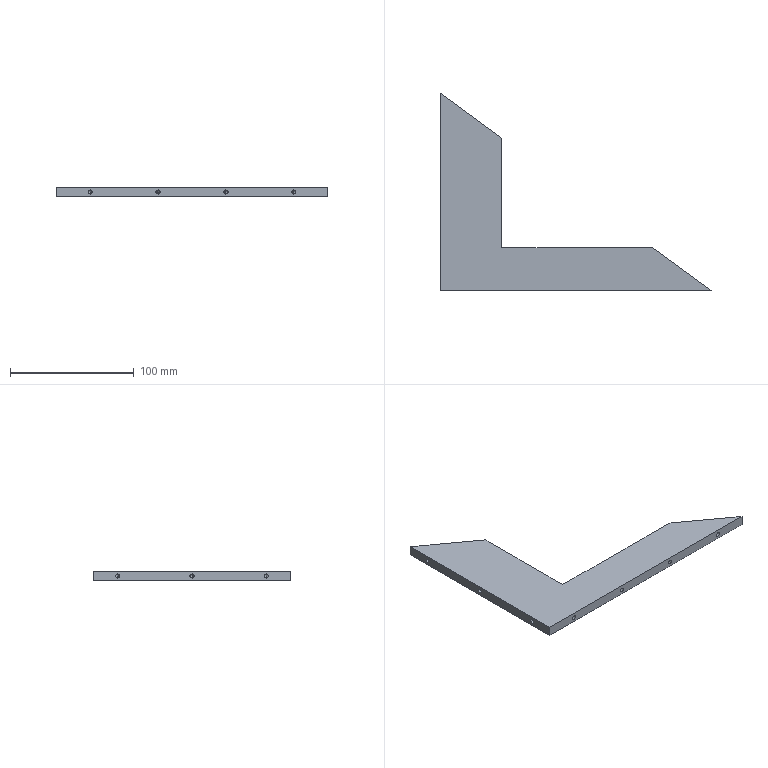Part | SolidWorks | features HoleWzd 2, Extrusion 1 | 1 solid | 36 faces | box 220 x 160 x 8 mm | volume 96669 mm3 | cylinder 14 | cone 14 | plane 8 | commonest cylinder face diameters 3.3 x14
STEP:
#1=CARTESIAN_POINT('',(-124.9,20.,2.35));
#2=VERTEX_POINT('',#1);
#3=CARTESIAN_POINT('',(-124.9,20.,5.65));
#4=VERTEX_POINT('',#3);
#5=CARTESIAN_POINT('',(-124.9,20.,4.));
#6=DIRECTION('',(-1.,0.,0.));
#7=DIRECTION('',(0.,0.,1.));
#8=AXIS2_PLACEMENT_3D('',#5,#6,#7);
#9=CIRCLE('',#8,1.65);
#10=EDGE_CURVE('',#2,#4,#9,.T.);
#11=ORIENTED_EDGE('',*,*,#10,.F.);
#12=CARTESIAN_POINT('',(-140.,20.,2.35));
#13=VERTEX_POINT('',#12);
#14=CARTESIAN_POINT('',(-140.,20.,2.35));
#15=DIRECTION('',(-1.,0.,0.));
#16=VECTOR('',#15,1000.);
#17=LINE('',#14,#16);
#18=EDGE_CURVE('',#2,#13,#17,.T.);
#19=ORIENTED_EDGE('',*,*,#18,.T.);
#20=CARTESIAN_POINT('',(-140.,20.,5.65));
#21=VERTEX_POINT('',#20);
#22=CARTESIAN_POINT('',(-140.,20.,4.));
#23=DIRECTION('',(-1.,0.,0.));
#24=DIRECTION('',(0.,0.,1.));
#25=AXIS2_PLACEMENT_3D('',#22,#23,#24);
#26=CIRCLE('',#25,1.65);
#27=EDGE_CURVE('',#13,#21,#26,.T.);
#28=ORIENTED_EDGE('',*,*,#27,.T.);
#29=CARTESIAN_POINT('',(-140.,20.,5.65));
#30=DIRECTION('',(-1.,0.,0.));
#31=VECTOR('',#30,1000.);
#32=LINE('',#29,#31);
#33=EDGE_CURVE('',#4,#21,#32,.T.);
#34=ORIENTED_EDGE('',*,*,#33,.F.);
#35=EDGE_LOOP('',(#11,#19,#28,#34));
#36=FACE_OUTER_BOUND('',#35,.T.);
#37=CARTESIAN_POINT('',(-140.,20.,4.));
#38=DIRECTION('',(-1.,0.,0.));
#39=DIRECTION('',(0.,0.,1.));
#40=AXIS2_PLACEMENT_3D('',#37,#38,#39);
#41=CYLINDRICAL_SURFACE('',#40,1.65);
#42=ADVANCED_FACE('',(#36),#41,.F.);
#43=CARTESIAN_POINT('',(-123.909,20.,4.));
#44=VERTEX_POINT('',#43);
#45=CARTESIAN_POINT('',(-124.9,20.,5.65));
#46=DIRECTION('',(-0.515,0.,0.8572));
#47=VECTOR('',#46,1000.);
#48=LINE('',#45,#47);
#49=EDGE_CURVE('',#44,#4,#48,.T.);
#50=ORIENTED_EDGE('',*,*,#49,.F.);
#51=CARTESIAN_POINT('',(-124.9,20.,2.35));
#52=DIRECTION('',(-0.515,0.,-0.8572));
#53=VECTOR('',#52,1000.);
#54=LINE('',#51,#53);
#55=EDGE_CURVE('',#44,#2,#54,.T.);
#56=ORIENTED_EDGE('',*,*,#55,.T.);
#57=ORIENTED_EDGE('',*,*,#10,.T.);
#58=EDGE_LOOP('',(#50,#56,#57));
#59=FACE_OUTER_BOUND('',#58,.T.);
#60=CARTESIAN_POINT('',(-124.9,20.,4.));
#61=DIRECTION('',(-1.,0.,0.));
#62=DIRECTION('',(0.,0.,1.));
#63=AXIS2_PLACEMENT_3D('',#60,#61,#62);
#64=CONICAL_SURFACE('',#63,1.65,1.03);
#65=ADVANCED_FACE('',(#59),#64,.F.);
#66=CARTESIAN_POINT('',(-124.9,-40.,2.35));
#67=VERTEX_POINT('',#66);
#68=CARTESIAN_POINT('',(-124.9,-40.,5.65));
#69=VERTEX_POINT('',#68);
#70=CARTESIAN_POINT('',(-124.9,-40.,4.));
#71=DIRECTION('',(-1.,0.,0.));
#72=DIRECTION('',(0.,0.,1.));
#73=AXIS2_PLACEMENT_3D('',#70,#71,#72);
#74=CIRCLE('',#73,1.65);
#75=EDGE_CURVE('',#67,#69,#74,.T.);
#76=ORIENTED_EDGE('',*,*,#75,.F.);
#77=CARTESIAN_POINT('',(-140.,-40.,2.35));
#78=VERTEX_POINT('',#77);
#79=CARTESIAN_POINT('',(-140.,-40.,2.35));
#80=DIRECTION('',(-1.,0.,0.));
#81=VECTOR('',#80,1000.);
#82=LINE('',#79,#81);
#83=EDGE_CURVE('',#67,#78,#82,.T.);
#84=ORIENTED_EDGE('',*,*,#83,.T.);
#85=CARTESIAN_POINT('',(-140.,-40.,5.65));
#86=VERTEX_POINT('',#85);
#87=CARTESIAN_POINT('',(-140.,-40.,4.));
#88=DIRECTION('',(-1.,0.,0.));
#89=DIRECTION('',(0.,0.,1.));
#90=AXIS2_PLACEMENT_3D('',#87,#88,#89);
#91=CIRCLE('',#90,1.65);
#92=EDGE_CURVE('',#78,#86,#91,.T.);
#93=ORIENTED_EDGE('',*,*,#92,.T.);
#94=CARTESIAN_POINT('',(-140.,-40.,5.65));
#95=DIRECTION('',(-1.,0.,0.));
#96=VECTOR('',#95,1000.);
#97=LINE('',#94,#96);
#98=EDGE_CURVE('',#69,#86,#97,.T.);
#99=ORIENTED_EDGE('',*,*,#98,.F.);
#100=EDGE_LOOP('',(#76,#84,#93,#99));
#101=FACE_OUTER_BOUND('',#100,.T.);
#102=CARTESIAN_POINT('',(-140.,-40.,4.));
#103=DIRECTION('',(-1.,0.,0.));
#104=DIRECTION('',(0.,0.,1.));
#105=AXIS2_PLACEMENT_3D('',#102,#103,#104);
#106=CYLINDRICAL_SURFACE('',#105,1.65);
#107=ADVANCED_FACE('',(#101),#106,.F.);
#108=CARTESIAN_POINT('',(-123.909,-40.,4.));
#109=VERTEX_POINT('',#108);
#110=CARTESIAN_POINT('',(-124.9,-40.,5.65));
#111=DIRECTION('',(-0.515,0.,0.8572));
#112=VECTOR('',#111,1000.);
#113=LINE('',#110,#112);
#114=EDGE_CURVE('',#109,#69,#113,.T.);
#115=ORIENTED_EDGE('',*,*,#114,.F.);
#116=CARTESIAN_POINT('',(-124.9,-40.,2.35));
#117=DIRECTION('',(-0.515,0.,-0.8572));
#118=VECTOR('',#117,1000.);
#119=LINE('',#116,#118);
#120=EDGE_CURVE('',#109,#67,#119,.T.);
#121=ORIENTED_EDGE('',*,*,#120,.T.);
#122=ORIENTED_EDGE('',*,*,#75,.T.);
#123=EDGE_LOOP('',(#115,#121,#122));
#124=FACE_OUTER_BOUND('',#123,.T.);
#125=CARTESIAN_POINT('',(-124.9,-40.,4.));
#126=DIRECTION('',(-1.,0.,0.));
#127=DIRECTION('',(0.,0.,1.));
#128=AXIS2_PLACEMENT_3D('',#125,#126,#127);
#129=CONICAL_SURFACE('',#128,1.65,1.03);
#130=ADVANCED_FACE('',(#124),#129,.F.);
#131=CARTESIAN_POINT('',(-124.9,-100.,2.35));
#132=VERTEX_POINT('',#131);
#133=CARTESIAN_POINT('',(-124.9,-100.,5.65));
#134=VERTEX_POINT('',#133);
#135=CARTESIAN_POINT('',(-124.9,-100.,4.));
#136=DIRECTION('',(-1.,0.,0.));
#137=DIRECTION('',(0.,0.,1.));
#138=AXIS2_PLACEMENT_3D('',#135,#136,#137);
#139=CIRCLE('',#138,1.65);
#140=EDGE_CURVE('',#132,#134,#139,.T.);
#141=ORIENTED_EDGE('',*,*,#140,.F.);
#142=CARTESIAN_POINT('',(-140.,-100.,2.35));
#143=VERTEX_POINT('',#142);
#144=CARTESIAN_POINT('',(-140.,-100.,2.35));
#145=DIRECTION('',(-1.,0.,0.));
#146=VECTOR('',#145,1000.);
#147=LINE('',#144,#146);
#148=EDGE_CURVE('',#132,#143,#147,.T.);
#149=ORIENTED_EDGE('',*,*,#148,.T.);
#150=CARTESIAN_POINT('',(-140.,-100.,5.65));
#151=VERTEX_POINT('',#150);
#152=CARTESIAN_POINT('',(-140.,-100.,4.));
#153=DIRECTION('',(-1.,0.,0.));
#154=DIRECTION('',(0.,0.,1.));
#155=AXIS2_PLACEMENT_3D('',#152,#153,#154);
#156=CIRCLE('',#155,1.65);
#157=EDGE_CURVE('',#143,#151,#156,.T.);
#158=ORIENTED_EDGE('',*,*,#157,.T.);
#159=CARTESIAN_POINT('',(-140.,-100.,5.65));
#160=DIRECTION('',(-1.,0.,0.));
#161=VECTOR('',#160,1000.);
#162=LINE('',#159,#161);
#163=EDGE_CURVE('',#134,#151,#162,.T.);
#164=ORIENTED_EDGE('',*,*,#163,.F.);
#165=EDGE_LOOP('',(#141,#149,#158,#164));
#166=FACE_OUTER_BOUND('',#165,.T.);
#167=CARTESIAN_POINT('',(-140.,-100.,4.));
#168=DIRECTION('',(-1.,0.,0.));
#169=DIRECTION('',(0.,0.,1.));
#170=AXIS2_PLACEMENT_3D('',#167,#168,#169);
#171=CYLINDRICAL_SURFACE('',#170,1.65);
#172=ADVANCED_FACE('',(#166),#171,.F.);
#173=CARTESIAN_POINT('',(-123.909,-100.,4.));
#174=VERTEX_POINT('',#173);
#175=CARTESIAN_POINT('',(-124.9,-100.,5.65));
#176=DIRECTION('',(-0.515,0.,0.8572));
#177=VECTOR('',#176,1000.);
#178=LINE('',#175,#177);
#179=EDGE_CURVE('',#174,#134,#178,.T.);
#180=ORIENTED_EDGE('',*,*,#179,.F.);
#181=CARTESIAN_POINT('',(-124.9,-100.,2.35));
#182=DIRECTION('',(-0.515,0.,-0.8572));
#183=VECTOR('',#182,1000.);
#184=LINE('',#181,#183);
#185=EDGE_CURVE('',#174,#132,#184,.T.);
#186=ORIENTED_EDGE('',*,*,#185,.T.);
#187=ORIENTED_EDGE('',*,*,#140,.T.);
#188=EDGE_LOOP('',(#180,#186,#187));
#189=FACE_OUTER_BOUND('',#188,.T.);
#190=CARTESIAN_POINT('',(-124.9,-100.,4.));
#191=DIRECTION('',(-1.,0.,0.));
#192=DIRECTION('',(0.,0.,1.));
#193=AXIS2_PLACEMENT_3D('',#190,#191,#192);
#194=CONICAL_SURFACE('',#193,1.65,1.03);
#195=ADVANCED_FACE('',(#189),#194,.F.);
#196=CARTESIAN_POINT('',(-112.5,-105.,5.65));
#197=VERTEX_POINT('',#196);
#198=CARTESIAN_POINT('',(-112.5,-105.,2.35));
#199=VERTEX_POINT('',#198);
#200=CARTESIAN_POINT('',(-112.5,-105.,4.));
#201=DIRECTION('',(0.,-1.,0.));
#202=DIRECTION('',(0.,0.,-1.));
#203=AXIS2_PLACEMENT_3D('',#200,#201,#202);
#204=CIRCLE('',#203,1.65);
#205=EDGE_CURVE('',#197,#199,#204,.T.);
#206=ORIENTED_EDGE('',*,*,#205,.F.);
#207=CARTESIAN_POINT('',(-112.5,-120.,5.65));
#208=VERTEX_POINT('',#207);
#209=CARTESIAN_POINT('',(-112.5,-120.,5.65));
#210=DIRECTION('',(0.,-1.,0.));
#211=VECTOR('',#210,1000.);
#212=LINE('',#209,#211);
#213=EDGE_CURVE('',#197,#208,#212,.T.);
#214=ORIENTED_EDGE('',*,*,#213,.T.);
#215=CARTESIAN_POINT('',(-112.5,-120.,2.35));
#216=VERTEX_POINT('',#215);
#217=CARTESIAN_POINT('',(-112.5,-120.,4.));
#218=DIRECTION('',(0.,-1.,0.));
#219=DIRECTION('',(0.,0.,-1.));
#220=AXIS2_PLACEMENT_3D('',#217,#218,#219);
#221=CIRCLE('',#220,1.65);
#222=EDGE_CURVE('',#208,#216,#221,.T.);
#223=ORIENTED_EDGE('',*,*,#222,.T.);
#224=CARTESIAN_POINT('',(-112.5,-120.,2.35));
#225=DIRECTION('',(0.,-1.,0.));
#226=VECTOR('',#225,1000.);
#227=LINE('',#224,#226);
#228=EDGE_CURVE('',#199,#216,#227,.T.);
#229=ORIENTED_EDGE('',*,*,#228,.F.);
#230=EDGE_LOOP('',(#206,#214,#223,#229));
#231=FACE_OUTER_BOUND('',#230,.T.);
#232=CARTESIAN_POINT('',(-112.5,-120.,4.));
#233=DIRECTION('',(0.,-1.,0.));
#234=DIRECTION('',(0.,0.,-1.));
#235=AXIS2_PLACEMENT_3D('',#232,#233,#234);
#236=CYLINDRICAL_SURFACE('',#235,1.65);
#237=ADVANCED_FACE('',(#231),#236,.F.);
#238=CARTESIAN_POINT('',(-112.5,-104.009,4.));
#239=VERTEX_POINT('',#238);
#240=CARTESIAN_POINT('',(-112.5,-105.,2.35));
#241=DIRECTION('',(0.,-0.515,-0.8572));
#242=VECTOR('',#241,1000.);
#243=LINE('',#240,#242);
#244=EDGE_CURVE('',#239,#199,#243,.T.);
#245=ORIENTED_EDGE('',*,*,#244,.F.);
#246=CARTESIAN_POINT('',(-112.5,-105.,5.65));
#247=DIRECTION('',(0.,-0.515,0.8572));
#248=VECTOR('',#247,1000.);
#249=LINE('',#246,#248);
#250=EDGE_CURVE('',#239,#197,#249,.T.);
#251=ORIENTED_EDGE('',*,*,#250,.T.);
#252=ORIENTED_EDGE('',*,*,#205,.T.);
#253=EDGE_LOOP('',(#245,#251,#252));
#254=FACE_OUTER_BOUND('',#253,.T.);
#255=CARTESIAN_POINT('',(-112.5,-105.,4.));
#256=DIRECTION('',(0.,-1.,0.));
#257=DIRECTION('',(0.,0.,-1.));
#258=AXIS2_PLACEMENT_3D('',#255,#256,#257);
#259=CONICAL_SURFACE('',#258,1.65,1.03);
#260=ADVANCED_FACE('',(#254),#259,.F.);
#261=CARTESIAN_POINT('',(-57.5,-105.,5.65));
#262=VERTEX_POINT('',#261);
#263=CARTESIAN_POINT('',(-57.5,-105.,2.35));
#264=VERTEX_POINT('',#263);
#265=CARTESIAN_POINT('',(-57.5,-105.,4.));
#266=DIRECTION('',(0.,-1.,0.));
#267=DIRECTION('',(0.,0.,-1.));
#268=AXIS2_PLACEMENT_3D('',#265,#266,#267);
#269=CIRCLE('',#268,1.65);
#270=EDGE_CURVE('',#262,#264,#269,.T.);
#271=ORIENTED_EDGE('',*,*,#270,.F.);
#272=CARTESIAN_POINT('',(-57.5,-120.,5.65));
#273=VERTEX_POINT('',#272);
#274=CARTESIAN_POINT('',(-57.5,-120.,5.65));
#275=DIRECTION('',(0.,-1.,0.));
#276=VECTOR('',#275,1000.);
#277=LINE('',#274,#276);
#278=EDGE_CURVE('',#262,#273,#277,.T.);
#279=ORIENTED_EDGE('',*,*,#278,.T.);
#280=CARTESIAN_POINT('',(-57.5,-120.,2.35));
#281=VERTEX_POINT('',#280);
#282=CARTESIAN_POINT('',(-57.5,-120.,4.));
#283=DIRECTION('',(0.,-1.,0.));
#284=DIRECTION('',(0.,0.,-1.));
#285=AXIS2_PLACEMENT_3D('',#282,#283,#284);
#286=CIRCLE('',#285,1.65);
#287=EDGE_CURVE('',#273,#281,#286,.T.);
#288=ORIENTED_EDGE('',*,*,#287,.T.);
#289=CARTESIAN_POINT('',(-57.5,-120.,2.35));
#290=DIRECTION('',(0.,-1.,0.));
#291=VECTOR('',#290,1000.);
#292=LINE('',#289,#291);
#293=EDGE_CURVE('',#264,#281,#292,.T.);
#294=ORIENTED_EDGE('',*,*,#293,.F.);
#295=EDGE_LOOP('',(#271,#279,#288,#294));
#296=FACE_OUTER_BOUND('',#295,.T.);
#297=CARTESIAN_POINT('',(-57.5,-120.,4.));
#298=DIRECTION('',(0.,-1.,0.));
#299=DIRECTION('',(0.,0.,-1.));
#300=AXIS2_PLACEMENT_3D('',#297,#298,#299);
#301=CYLINDRICAL_SURFACE('',#300,1.65);
#302=ADVANCED_FACE('',(#296),#301,.F.);
#303=CARTESIAN_POINT('',(-57.5,-104.009,4.));
#304=VERTEX_POINT('',#303);
#305=CARTESIAN_POINT('',(-57.5,-105.,2.35));
#306=DIRECTION('',(0.,-0.515,-0.8572));
#307=VECTOR('',#306,1000.);
#308=LINE('',#305,#307);
#309=EDGE_CURVE('',#304,#264,#308,.T.);
#310=ORIENTED_EDGE('',*,*,#309,.F.);
#311=CARTESIAN_POINT('',(-57.5,-105.,5.65));
#312=DIRECTION('',(0.,-0.515,0.8572));
#313=VECTOR('',#312,1000.);
#314=LINE('',#311,#313);
#315=EDGE_CURVE('',#304,#262,#314,.T.);
#316=ORIENTED_EDGE('',*,*,#315,.T.);
#317=ORIENTED_EDGE('',*,*,#270,.T.);
#318=EDGE_LOOP('',(#310,#316,#317));
#319=FACE_OUTER_BOUND('',#318,.T.);
#320=CARTESIAN_POINT('',(-57.5,-105.,4.));
#321=DIRECTION('',(0.,-1.,0.));
#322=DIRECTION('',(0.,0.,-1.));
#323=AXIS2_PLACEMENT_3D('',#320,#321,#322);
#324=CONICAL_SURFACE('',#323,1.65,1.03);
#325=ADVANCED_FACE('',(#319),#324,.F.);
#326=CARTESIAN_POINT('',(-2.5,-105.,5.65));
#327=VERTEX_POINT('',#326);
#328=CARTESIAN_POINT('',(-2.5,-105.,2.35));
#329=VERTEX_POINT('',#328);
#330=CARTESIAN_POINT('',(-2.5,-105.,4.));
#331=DIRECTION('',(0.,-1.,0.));
#332=DIRECTION('',(0.,0.,-1.));
#333=AXIS2_PLACEMENT_3D('',#330,#331,#332);
#334=CIRCLE('',#333,1.65);
#335=EDGE_CURVE('',#327,#329,#334,.T.);
#336=ORIENTED_EDGE('',*,*,#335,.F.);
#337=CARTESIAN_POINT('',(-2.5,-120.,5.65));
#338=VERTEX_POINT('',#337);
#339=CARTESIAN_POINT('',(-2.5,-120.,5.65));
#340=DIRECTION('',(0.,-1.,0.));
#341=VECTOR('',#340,1000.);
#342=LINE('',#339,#341);
#343=EDGE_CURVE('',#327,#338,#342,.T.);
#344=ORIENTED_EDGE('',*,*,#343,.T.);
#345=CARTESIAN_POINT('',(-2.5,-120.,2.35));
#346=VERTEX_POINT('',#345);
#347=CARTESIAN_POINT('',(-2.5,-120.,4.));
#348=DIRECTION('',(0.,-1.,0.));
#349=DIRECTION('',(0.,0.,-1.));
#350=AXIS2_PLACEMENT_3D('',#347,#348,#349);
#351=CIRCLE('',#350,1.65);
#352=EDGE_CURVE('',#338,#346,#351,.T.);
#353=ORIENTED_EDGE('',*,*,#352,.T.);
#354=CARTESIAN_POINT('',(-2.5,-120.,2.35));
#355=DIRECTION('',(0.,-1.,0.));
#356=VECTOR('',#355,1000.);
#357=LINE('',#354,#356);
#358=EDGE_CURVE('',#329,#346,#357,.T.);
#359=ORIENTED_EDGE('',*,*,#358,.F.);
#360=EDGE_LOOP('',(#336,#344,#353,#359));
#361=FACE_OUTER_BOUND('',#360,.T.);
#362=CARTESIAN_POINT('',(-2.5,-120.,4.));
#363=DIRECTION('',(0.,-1.,0.));
#364=DIRECTION('',(0.,0.,-1.));
#365=AXIS2_PLACEMENT_3D('',#362,#363,#364);
#366=CYLINDRICAL_SURFACE('',#365,1.65);
#367=ADVANCED_FACE('',(#361),#366,.F.);
#368=CARTESIAN_POINT('',(-2.5,-104.009,4.));
#369=VERTEX_POINT('',#368);
#370=CARTESIAN_POINT('',(-2.5,-105.,2.35));
#371=DIRECTION('',(0.,-0.515,-0.8572));
#372=VECTOR('',#371,1000.);
#373=LINE('',#370,#372);
#374=EDGE_CURVE('',#369,#329,#373,.T.);
#375=ORIENTED_EDGE('',*,*,#374,.F.);
#376=CARTESIAN_POINT('',(-2.5,-105.,5.65));
#377=DIRECTION('',(0.,-0.515,0.8572));
#378=VECTOR('',#377,1000.);
#379=LINE('',#376,#378);
#380=EDGE_CURVE('',#369,#327,#379,.T.);
#381=ORIENTED_EDGE('',*,*,#380,.T.);
#382=ORIENTED_EDGE('',*,*,#335,.T.);
#383=EDGE_LOOP('',(#375,#381,#382));
#384=FACE_OUTER_BOUND('',#383,.T.);
#385=CARTESIAN_POINT('',(-2.5,-105.,4.));
#386=DIRECTION('',(0.,-1.,0.));
#387=DIRECTION('',(0.,0.,-1.));
#388=AXIS2_PLACEMENT_3D('',#385,#386,#387);
#389=CONICAL_SURFACE('',#388,1.65,1.03);
#390=ADVANCED_FACE('',(#384),#389,.F.);
#391=CARTESIAN_POINT('',(52.5,-105.,5.65));
#392=VERTEX_POINT('',#391);
#393=CARTESIAN_POINT('',(52.5,-105.,2.35));
#394=VERTEX_POINT('',#393);
#395=CARTESIAN_POINT('',(52.5,-105.,4.));
#396=DIRECTION('',(0.,-1.,0.));
#397=DIRECTION('',(0.,0.,-1.));
#398=AXIS2_PLACEMENT_3D('',#395,#396,#397);
#399=CIRCLE('',#398,1.65);
#400=EDGE_CURVE('',#392,#394,#399,.T.);
#401=ORIENTED_EDGE('',*,*,#400,.F.);
#402=CARTESIAN_POINT('',(52.5,-120.,5.65));
#403=VERTEX_POINT('',#402);
#404=CARTESIAN_POINT('',(52.5,-120.,5.65));
#405=DIRECTION('',(0.,-1.,0.));
#406=VECTOR('',#405,1000.);
#407=LINE('',#404,#406);
#408=EDGE_CURVE('',#392,#403,#407,.T.);
#409=ORIENTED_EDGE('',*,*,#408,.T.);
#410=CARTESIAN_POINT('',(52.5,-120.,2.35));
#411=VERTEX_POINT('',#410);
#412=CARTESIAN_POINT('',(52.5,-120.,4.));
#413=DIRECTION('',(0.,-1.,0.));
#414=DIRECTION('',(0.,0.,-1.));
#415=AXIS2_PLACEMENT_3D('',#412,#413,#414);
#416=CIRCLE('',#415,1.65);
#417=EDGE_CURVE('',#403,#411,#416,.T.);
#418=ORIENTED_EDGE('',*,*,#417,.T.);
#419=CARTESIAN_POINT('',(52.5,-120.,2.35));
#420=DIRECTION('',(0.,-1.,0.));
#421=VECTOR('',#420,1000.);
#422=LINE('',#419,#421);
#423=EDGE_CURVE('',#394,#411,#422,.T.);
#424=ORIENTED_EDGE('',*,*,#423,.F.);
#425=EDGE_LOOP('',(#401,#409,#418,#424));
#426=FACE_OUTER_BOUND('',#425,.T.);
#427=CARTESIAN_POINT('',(52.5,-120.,4.));
#428=DIRECTION('',(0.,-1.,0.));
#429=DIRECTION('',(0.,0.,-1.));
#430=AXIS2_PLACEMENT_3D('',#427,#428,#429);
#431=CYLINDRICAL_SURFACE('',#430,1.65);
#432=ADVANCED_FACE('',(#426),#431,.F.);
#433=CARTESIAN_POINT('',(52.5,-104.009,4.));
#434=VERTEX_POINT('',#433);
#435=CARTESIAN_POINT('',(52.5,-105.,2.35));
#436=DIRECTION('',(0.,-0.515,-0.8572));
#437=VECTOR('',#436,1000.);
#438=LINE('',#435,#437);
#439=EDGE_CURVE('',#434,#394,#438,.T.);
#440=ORIENTED_EDGE('',*,*,#439,.F.);
#441=CARTESIAN_POINT('',(52.5,-105.,5.65));
#442=DIRECTION('',(0.,-0.515,0.8572));
#443=VECTOR('',#442,1000.);
#444=LINE('',#441,#443);
#445=EDGE_CURVE('',#434,#392,#444,.T.);
#446=ORIENTED_EDGE('',*,*,#445,.T.);
#447=ORIENTED_EDGE('',*,*,#400,.T.);
#448=EDGE_LOOP('',(#440,#446,#447));
#449=FACE_OUTER_BOUND('',#448,.T.);
#450=CARTESIAN_POINT('',(52.5,-105.,4.));
#451=DIRECTION('',(0.,-1.,0.));
#452=DIRECTION('',(0.,0.,-1.));
#453=AXIS2_PLACEMENT_3D('',#450,#451,#452);
#454=CONICAL_SURFACE('',#453,1.65,1.03);
#455=ADVANCED_FACE('',(#449),#454,.F.);
#456=CARTESIAN_POINT('',(-90.,3.636,0.));
#457=VERTEX_POINT('',#456);
#458=CARTESIAN_POINT('',(-140.,40.,0.));
#459=VERTEX_POINT('',#458);
#460=CARTESIAN_POINT('',(-90.,3.636,0.));
#461=DIRECTION('',(-0.8087,0.5882,0.));
#462=VECTOR('',#461,1000.);
#463=LINE('',#460,#462);
#464=EDGE_CURVE('',#457,#459,#463,.T.);
#465=ORIENTED_EDGE('',*,*,#464,.T.);
#466=CARTESIAN_POINT('',(-140.,40.,8.));
#467=VERTEX_POINT('',#466);
#468=CARTESIAN_POINT('',(-140.,40.,8.));
#469=DIRECTION('',(0.,0.,-1.));
#470=VECTOR('',#469,1000.);
#471=LINE('',#468,#470);
#472=EDGE_CURVE('',#467,#459,#471,.T.);
#473=ORIENTED_EDGE('',*,*,#472,.F.);
#474=CARTESIAN_POINT('',(-90.,3.636,8.));
#475=VERTEX_POINT('',#474);
#476=CARTESIAN_POINT('',(-90.,3.636,8.));
#477=DIRECTION('',(-0.8087,0.5882,0.));
#478=VECTOR('',#477,1000.);
#479=LINE('',#476,#478);
#480=EDGE_CURVE('',#475,#467,#479,.T.);
#481=ORIENTED_EDGE('',*,*,#480,.F.);
#482=CARTESIAN_POINT('',(-90.,3.636,8.));
#483=DIRECTION('',(0.,0.,-1.));
#484=VECTOR('',#483,1000.);
#485=LINE('',#482,#484);
#486=EDGE_CURVE('',#475,#457,#485,.T.);
#487=ORIENTED_EDGE('',*,*,#486,.T.);
#488=EDGE_LOOP('',(#465,#473,#481,#487));
#489=FACE_OUTER_BOUND('',#488,.T.);
#490=CARTESIAN_POINT('',(-90.,3.636,8.));
#491=DIRECTION('',(-0.5882,-0.8087,0.));
#492=DIRECTION('',(0.8087,-0.5882,0.));
#493=AXIS2_PLACEMENT_3D('',#490,#491,#492);
#494=PLANE('',#493);
#495=ADVANCED_FACE('',(#489),#494,.F.);
#496=CARTESIAN_POINT('',(-140.,20.,4.));
#497=DIRECTION('',(-1.,0.,0.));
#498=DIRECTION('',(0.,0.,1.));
#499=AXIS2_PLACEMENT_3D('',#496,#497,#498);
#500=CIRCLE('',#499,1.65);
#501=EDGE_CURVE('',#21,#13,#500,.T.);
#502=ORIENTED_EDGE('',*,*,#501,.F.);
#503=ORIENTED_EDGE('',*,*,#27,.F.);
#504=EDGE_LOOP('',(#502,#503));
#505=FACE_BOUND('',#504,.T.);
#506=CARTESIAN_POINT('',(-140.,-40.,4.));
#507=DIRECTION('',(-1.,0.,0.));
#508=DIRECTION('',(0.,0.,1.));
#509=AXIS2_PLACEMENT_3D('',#506,#507,#508);
#510=CIRCLE('',#509,1.65);
#511=EDGE_CURVE('',#86,#78,#510,.T.);
#512=ORIENTED_EDGE('',*,*,#511,.F.);
#513=ORIENTED_EDGE('',*,*,#92,.F.);
#514=EDGE_LOOP('',(#512,#513));
#515=FACE_BOUND('',#514,.T.);
#516=CARTESIAN_POINT('',(-140.,-100.,4.));
#517=DIRECTION('',(-1.,0.,0.));
#518=DIRECTION('',(0.,0.,1.));
#519=AXIS2_PLACEMENT_3D('',#516,#517,#518);
#520=CIRCLE('',#519,1.65);
#521=EDGE_CURVE('',#151,#143,#520,.T.);
#522=ORIENTED_EDGE('',*,*,#521,.F.);
#523=ORIENTED_EDGE('',*,*,#157,.F.);
#524=EDGE_LOOP('',(#522,#523));
#525=FACE_BOUND('',#524,.T.);
#526=CARTESIAN_POINT('',(-140.,-120.,0.));
#527=VERTEX_POINT('',#526);
#528=CARTESIAN_POINT('',(-140.,40.,0.));
#529=DIRECTION('',(0.,-1.,0.));
#530=VECTOR('',#529,1000.);
#531=LINE('',#528,#530);
#532=EDGE_CURVE('',#459,#527,#531,.T.);
#533=ORIENTED_EDGE('',*,*,#532,.T.);
#534=CARTESIAN_POINT('',(-140.,-120.,8.));
#535=VERTEX_POINT('',#534);
#536=CARTESIAN_POINT('',(-140.,-120.,8.));
#537=DIRECTION('',(0.,0.,-1.));
#538=VECTOR('',#537,1000.);
#539=LINE('',#536,#538);
#540=EDGE_CURVE('',#535,#527,#539,.T.);
#541=ORIENTED_EDGE('',*,*,#540,.F.);
#542=CARTESIAN_POINT('',(-140.,40.,8.));
#543=DIRECTION('',(0.,-1.,0.));
#544=VECTOR('',#543,1000.);
#545=LINE('',#542,#544);
#546=EDGE_CURVE('',#467,#535,#545,.T.);
#547=ORIENTED_EDGE('',*,*,#546,.F.);
#548=ORIENTED_EDGE('',*,*,#472,.T.);
#549=EDGE_LOOP('',(#533,#541,#547,#548));
#550=FACE_OUTER_BOUND('',#549,.T.);
#551=CARTESIAN_POINT('',(-140.,40.,8.));
#552=DIRECTION('',(1.,0.,0.));
#553=DIRECTION('',(0.,0.,-1.));
#554=AXIS2_PLACEMENT_3D('',#551,#552,#553);
#555=PLANE('',#554);
#556=ADVANCED_FACE('',(#505,#515,#525,#550),#555,.F.);
#557=CARTESIAN_POINT('',(-112.5,-120.,4.));
#558=DIRECTION('',(0.,-1.,0.));
#559=DIRECTION('',(0.,0.,-1.));
#560=AXIS2_PLACEMENT_3D('',#557,#558,#559);
#561=CIRCLE('',#560,1.65);
#562=EDGE_CURVE('',#216,#208,#561,.T.);
#563=ORIENTED_EDGE('',*,*,#562,.F.);
#564=ORIENTED_EDGE('',*,*,#222,.F.);
#565=EDGE_LOOP('',(#563,#564));
#566=FACE_BOUND('',#565,.T.);
#567=CARTESIAN_POINT('',(-57.5,-120.,4.));
#568=DIRECTION('',(0.,-1.,0.));
#569=DIRECTION('',(0.,0.,-1.));
#570=AXIS2_PLACEMENT_3D('',#567,#568,#569);
#571=CIRCLE('',#570,1.65);
#572=EDGE_CURVE('',#281,#273,#571,.T.);
#573=ORIENTED_EDGE('',*,*,#572,.F.);
#574=ORIENTED_EDGE('',*,*,#287,.F.);
#575=EDGE_LOOP('',(#573,#574));
#576=FACE_BOUND('',#575,.T.);
#577=CARTESIAN_POINT('',(-2.5,-120.,4.));
#578=DIRECTION('',(0.,-1.,0.));
#579=DIRECTION('',(0.,0.,-1.));
#580=AXIS2_PLACEMENT_3D('',#577,#578,#579);
#581=CIRCLE('',#580,1.65);
#582=EDGE_CURVE('',#346,#338,#581,.T.);
#583=ORIENTED_EDGE('',*,*,#582,.F.);
#584=ORIENTED_EDGE('',*,*,#352,.F.);
#585=EDGE_LOOP('',(#583,#584));
#586=FACE_BOUND('',#585,.T.);
#587=CARTESIAN_POINT('',(52.5,-120.,4.));
#588=DIRECTION('',(0.,-1.,0.));
#589=DIRECTION('',(0.,0.,-1.));
#590=AXIS2_PLACEMENT_3D('',#587,#588,#589);
#591=CIRCLE('',#590,1.65);
#592=EDGE_CURVE('',#411,#403,#591,.T.);
#593=ORIENTED_EDGE('',*,*,#592,.F.);
#594=ORIENTED_EDGE('',*,*,#417,.F.);
#595=EDGE_LOOP('',(#593,#594));
#596=FACE_BOUND('',#595,.T.);
#597=CARTESIAN_POINT('',(80.,-120.,0.));
#598=VERTEX_POINT('',#597);
#599=CARTESIAN_POINT('',(-140.,-120.,0.));
#600=DIRECTION('',(1.,0.,0.));
#601=VECTOR('',#600,1000.);
#602=LINE('',#599,#601);
#603=EDGE_CURVE('',#527,#598,#602,.T.);
#604=ORIENTED_EDGE('',*,*,#603,.T.);
#605=CARTESIAN_POINT('',(80.,-120.,8.));
#606=VERTEX_POINT('',#605);
#607=CARTESIAN_POINT('',(80.,-120.,8.));
#608=DIRECTION('',(0.,0.,-1.));
#609=VECTOR('',#608,1000.);
#610=LINE('',#607,#609);
#611=EDGE_CURVE('',#606,#598,#610,.T.);
#612=ORIENTED_EDGE('',*,*,#611,.F.);
#613=CARTESIAN_POINT('',(-140.,-120.,8.));
#614=DIRECTION('',(1.,0.,0.));
#615=VECTOR('',#614,1000.);
#616=LINE('',#613,#615);
#617=EDGE_CURVE('',#535,#606,#616,.T.);
#618=ORIENTED_EDGE('',*,*,#617,.F.);
#619=ORIENTED_EDGE('',*,*,#540,.T.);
#620=EDGE_LOOP('',(#604,#612,#618,#619));
#621=FACE_OUTER_BOUND('',#620,.T.);
#622=CARTESIAN_POINT('',(-140.,-120.,8.));
#623=DIRECTION('',(0.,1.,0.));
#624=DIRECTION('',(-1.,0.,0.));
#625=AXIS2_PLACEMENT_3D('',#622,#623,#624);
#626=PLANE('',#625);
#627=ADVANCED_FACE('',(#566,#576,#586,#596,#621),#626,.F.);
#628=CARTESIAN_POINT('',(31.875,-85.,0.));
#629=VERTEX_POINT('',#628);
#630=CARTESIAN_POINT('',(80.,-120.,0.));
#631=DIRECTION('',(-0.8087,0.5882,0.));
#632=VECTOR('',#631,1000.);
#633=LINE('',#630,#632);
#634=EDGE_CURVE('',#598,#629,#633,.T.);
#635=ORIENTED_EDGE('',*,*,#634,.T.);
#636=CARTESIAN_POINT('',(31.875,-85.,8.));
#637=VERTEX_POINT('',#636);
#638=CARTESIAN_POINT('',(31.875,-85.,8.));
#639=DIRECTION('',(0.,0.,-1.));
#640=VECTOR('',#639,1000.);
#641=LINE('',#638,#640);
#642=EDGE_CURVE('',#637,#629,#641,.T.);
#643=ORIENTED_EDGE('',*,*,#642,.F.);
#644=CARTESIAN_POINT('',(80.,-120.,8.));
#645=DIRECTION('',(-0.8087,0.5882,0.));
#646=VECTOR('',#645,1000.);
#647=LINE('',#644,#646);
#648=EDGE_CURVE('',#606,#637,#647,.T.);
#649=ORIENTED_EDGE('',*,*,#648,.F.);
#650=ORIENTED_EDGE('',*,*,#611,.T.);
#651=EDGE_LOOP('',(#635,#643,#649,#650));
#652=FACE_OUTER_BOUND('',#651,.T.);
#653=CARTESIAN_POINT('',(80.,-120.,8.));
#654=DIRECTION('',(-0.5882,-0.8087,0.));
#655=DIRECTION('',(0.8087,-0.5882,0.));
#656=AXIS2_PLACEMENT_3D('',#653,#654,#655);
#657=PLANE('',#656);
#658=ADVANCED_FACE('',(#652),#657,.F.);
#659=CARTESIAN_POINT('',(-90.,-85.,0.));
#660=VERTEX_POINT('',#659);
#661=CARTESIAN_POINT('',(31.875,-85.,0.));
#662=DIRECTION('',(-1.,0.,0.));
#663=VECTOR('',#662,1000.);
#664=LINE('',#661,#663);
#665=EDGE_CURVE('',#629,#660,#664,.T.);
#666=ORIENTED_EDGE('',*,*,#665,.T.);
#667=CARTESIAN_POINT('',(-90.,-85.,8.));
#668=VERTEX_POINT('',#667);
#669=CARTESIAN_POINT('',(-90.,-85.,8.));
#670=DIRECTION('',(0.,0.,-1.));
#671=VECTOR('',#670,1000.);
#672=LINE('',#669,#671);
#673=EDGE_CURVE('',#668,#660,#672,.T.);
#674=ORIENTED_EDGE('',*,*,#673,.F.);
#675=CARTESIAN_POINT('',(31.875,-85.,8.));
#676=DIRECTION('',(-1.,0.,0.));
#677=VECTOR('',#676,1000.);
#678=LINE('',#675,#677);
#679=EDGE_CURVE('',#637,#668,#678,.T.);
#680=ORIENTED_EDGE('',*,*,#679,.F.);
#681=ORIENTED_EDGE('',*,*,#642,.T.);
#682=EDGE_LOOP('',(#666,#674,#680,#681));
#683=FACE_OUTER_BOUND('',#682,.T.);
#684=CARTESIAN_POINT('',(31.875,-85.,8.));
#685=DIRECTION('',(0.,-1.,0.));
#686=DIRECTION('',(1.,0.,0.));
#687=AXIS2_PLACEMENT_3D('',#684,#685,#686);
#688=PLANE('',#687);
#689=ADVANCED_FACE('',(#683),#688,.F.);
#690=CARTESIAN_POINT('',(-90.,-85.,0.));
#691=DIRECTION('',(0.,1.,0.));
#692=VECTOR('',#691,1000.);
#693=LINE('',#690,#692);
#694=EDGE_CURVE('',#660,#457,#693,.T.);
#695=ORIENTED_EDGE('',*,*,#694,.T.);
#696=ORIENTED_EDGE('',*,*,#486,.F.);
#697=CARTESIAN_POINT('',(-90.,-85.,8.));
#698=DIRECTION('',(0.,1.,0.));
#699=VECTOR('',#698,1000.);
#700=LINE('',#697,#699);
#701=EDGE_CURVE('',#668,#475,#700,.T.);
#702=ORIENTED_EDGE('',*,*,#701,.F.);
#703=ORIENTED_EDGE('',*,*,#673,.T.);
#704=EDGE_LOOP('',(#695,#696,#702,#703));
#705=FACE_OUTER_BOUND('',#704,.T.);
#706=CARTESIAN_POINT('',(-90.,-85.,8.));
#707=DIRECTION('',(-1.,0.,0.));
#708=DIRECTION('',(0.,-1.,0.));
#709=AXIS2_PLACEMENT_3D('',#706,#707,#708);
#710=PLANE('',#709);
#711=ADVANCED_FACE('',(#705),#710,.F.);
#712=ORIENTED_EDGE('',*,*,#480,.T.);
#713=ORIENTED_EDGE('',*,*,#546,.T.);
#714=ORIENTED_EDGE('',*,*,#617,.T.);
#715=ORIENTED_EDGE('',*,*,#648,.T.);
#716=ORIENTED_EDGE('',*,*,#679,.T.);
#717=ORIENTED_EDGE('',*,*,#701,.T.);
#718=EDGE_LOOP('',(#712,#713,#714,#715,#716,#717));
#719=FACE_OUTER_BOUND('',#718,.T.);
#720=CARTESIAN_POINT('',(0.,0.,8.));
#721=DIRECTION('',(0.,0.,1.));
#722=DIRECTION('',(1.,0.,0.));
#723=AXIS2_PLACEMENT_3D('',#720,#721,#722);
#724=PLANE('',#723);
#725=ADVANCED_FACE('',(#719),#724,.T.);
#726=ORIENTED_EDGE('',*,*,#464,.F.);
#727=ORIENTED_EDGE('',*,*,#694,.F.);
#728=ORIENTED_EDGE('',*,*,#665,.F.);
#729=ORIENTED_EDGE('',*,*,#634,.F.);
#730=ORIENTED_EDGE('',*,*,#603,.F.);
#731=ORIENTED_EDGE('',*,*,#532,.F.);
#732=EDGE_LOOP('',(#726,#727,#728,#729,#730,#731));
#733=FACE_OUTER_BOUND('',#732,.T.);
#734=CARTESIAN_POINT('',(0.,0.,0.));
#735=DIRECTION('',(0.,0.,1.));
#736=DIRECTION('',(1.,0.,0.));
#737=AXIS2_PLACEMENT_3D('',#734,#735,#736);
#738=PLANE('',#737);
#739=ADVANCED_FACE('',(#733),#738,.F.);
#740=ORIENTED_EDGE('',*,*,#445,.F.);
#741=ORIENTED_EDGE('',*,*,#439,.T.);
#742=CARTESIAN_POINT('',(52.5,-105.,4.));
#743=DIRECTION('',(0.,-1.,0.));
#744=DIRECTION('',(0.,0.,-1.));
#745=AXIS2_PLACEMENT_3D('',#742,#743,#744);
#746=CIRCLE('',#745,1.65);
#747=EDGE_CURVE('',#394,#392,#746,.T.);
#748=ORIENTED_EDGE('',*,*,#747,.T.);
#749=EDGE_LOOP('',(#740,#741,#748));
#750=FACE_OUTER_BOUND('',#749,.T.);
#751=CARTESIAN_POINT('',(52.5,-105.,4.));
#752=DIRECTION('',(0.,-1.,0.));
#753=DIRECTION('',(0.,0.,-1.));
#754=AXIS2_PLACEMENT_3D('',#751,#752,#753);
#755=CONICAL_SURFACE('',#754,1.65,1.03);
#756=ADVANCED_FACE('',(#750),#755,.F.);
#757=ORIENTED_EDGE('',*,*,#408,.F.);
#758=ORIENTED_EDGE('',*,*,#747,.F.);
#759=ORIENTED_EDGE('',*,*,#423,.T.);
#760=ORIENTED_EDGE('',*,*,#592,.T.);
#761=EDGE_LOOP('',(#757,#758,#759,#760));
#762=FACE_OUTER_BOUND('',#761,.T.);
#763=CARTESIAN_POINT('',(52.5,-120.,4.));
#764=DIRECTION('',(0.,-1.,0.));
#765=DIRECTION('',(0.,0.,-1.));
#766=AXIS2_PLACEMENT_3D('',#763,#764,#765);
#767=CYLINDRICAL_SURFACE('',#766,1.65);
#768=ADVANCED_FACE('',(#762),#767,.F.);
#769=ORIENTED_EDGE('',*,*,#380,.F.);
#770=ORIENTED_EDGE('',*,*,#374,.T.);
#771=CARTESIAN_POINT('',(-2.5,-105.,4.));
#772=DIRECTION('',(0.,-1.,0.));
#773=DIRECTION('',(0.,0.,-1.));
#774=AXIS2_PLACEMENT_3D('',#771,#772,#773);
#775=CIRCLE('',#774,1.65);
#776=EDGE_CURVE('',#329,#327,#775,.T.);
#777=ORIENTED_EDGE('',*,*,#776,.T.);
#778=EDGE_LOOP('',(#769,#770,#777));
#779=FACE_OUTER_BOUND('',#778,.T.);
#780=CARTESIAN_POINT('',(-2.5,-105.,4.));
#781=DIRECTION('',(0.,-1.,0.));
#782=DIRECTION('',(0.,0.,-1.));
#783=AXIS2_PLACEMENT_3D('',#780,#781,#782);
#784=CONICAL_SURFACE('',#783,1.65,1.03);
#785=ADVANCED_FACE('',(#779),#784,.F.);
#786=ORIENTED_EDGE('',*,*,#343,.F.);
#787=ORIENTED_EDGE('',*,*,#776,.F.);
#788=ORIENTED_EDGE('',*,*,#358,.T.);
#789=ORIENTED_EDGE('',*,*,#582,.T.);
#790=EDGE_LOOP('',(#786,#787,#788,#789));
#791=FACE_OUTER_BOUND('',#790,.T.);
#792=CARTESIAN_POINT('',(-2.5,-120.,4.));
#793=DIRECTION('',(0.,-1.,0.));
#794=DIRECTION('',(0.,0.,-1.));
#795=AXIS2_PLACEMENT_3D('',#792,#793,#794);
#796=CYLINDRICAL_SURFACE('',#795,1.65);
#797=ADVANCED_FACE('',(#791),#796,.F.);
#798=ORIENTED_EDGE('',*,*,#315,.F.);
#799=ORIENTED_EDGE('',*,*,#309,.T.);
#800=CARTESIAN_POINT('',(-57.5,-105.,4.));
#801=DIRECTION('',(0.,-1.,0.));
#802=DIRECTION('',(0.,0.,-1.));
#803=AXIS2_PLACEMENT_3D('',#800,#801,#802);
#804=CIRCLE('',#803,1.65);
#805=EDGE_CURVE('',#264,#262,#804,.T.);
#806=ORIENTED_EDGE('',*,*,#805,.T.);
#807=EDGE_LOOP('',(#798,#799,#806));
#808=FACE_OUTER_BOUND('',#807,.T.);
#809=CARTESIAN_POINT('',(-57.5,-105.,4.));
#810=DIRECTION('',(0.,-1.,0.));
#811=DIRECTION('',(0.,0.,-1.));
#812=AXIS2_PLACEMENT_3D('',#809,#810,#811);
#813=CONICAL_SURFACE('',#812,1.65,1.03);
#814=ADVANCED_FACE('',(#808),#813,.F.);
#815=ORIENTED_EDGE('',*,*,#278,.F.);
#816=ORIENTED_EDGE('',*,*,#805,.F.);
#817=ORIENTED_EDGE('',*,*,#293,.T.);
#818=ORIENTED_EDGE('',*,*,#572,.T.);
#819=EDGE_LOOP('',(#815,#816,#817,#818));
#820=FACE_OUTER_BOUND('',#819,.T.);
#821=CARTESIAN_POINT('',(-57.5,-120.,4.));
#822=DIRECTION('',(0.,-1.,0.));
#823=DIRECTION('',(0.,0.,-1.));
#824=AXIS2_PLACEMENT_3D('',#821,#822,#823);
#825=CYLINDRICAL_SURFACE('',#824,1.65);
#826=ADVANCED_FACE('',(#820),#825,.F.);
#827=ORIENTED_EDGE('',*,*,#250,.F.);
#828=ORIENTED_EDGE('',*,*,#244,.T.);
#829=CARTESIAN_POINT('',(-112.5,-105.,4.));
#830=DIRECTION('',(0.,-1.,0.));
#831=DIRECTION('',(0.,0.,-1.));
#832=AXIS2_PLACEMENT_3D('',#829,#830,#831);
#833=CIRCLE('',#832,1.65);
#834=EDGE_CURVE('',#199,#197,#833,.T.);
#835=ORIENTED_EDGE('',*,*,#834,.T.);
#836=EDGE_LOOP('',(#827,#828,#835));
#837=FACE_OUTER_BOUND('',#836,.T.);
#838=CARTESIAN_POINT('',(-112.5,-105.,4.));
#839=DIRECTION('',(0.,-1.,0.));
#840=DIRECTION('',(0.,0.,-1.));
#841=AXIS2_PLACEMENT_3D('',#838,#839,#840);
#842=CONICAL_SURFACE('',#841,1.65,1.03);
#843=ADVANCED_FACE('',(#837),#842,.F.);
#844=ORIENTED_EDGE('',*,*,#213,.F.);
#845=ORIENTED_EDGE('',*,*,#834,.F.);
#846=ORIENTED_EDGE('',*,*,#228,.T.);
#847=ORIENTED_EDGE('',*,*,#562,.T.);
#848=EDGE_LOOP('',(#844,#845,#846,#847));
#849=FACE_OUTER_BOUND('',#848,.T.);
#850=CARTESIAN_POINT('',(-112.5,-120.,4.));
#851=DIRECTION('',(0.,-1.,0.));
#852=DIRECTION('',(0.,0.,-1.));
#853=AXIS2_PLACEMENT_3D('',#850,#851,#852);
#854=CYLINDRICAL_SURFACE('',#853,1.65);
#855=ADVANCED_FACE('',(#849),#854,.F.);
#856=ORIENTED_EDGE('',*,*,#185,.F.);
#857=ORIENTED_EDGE('',*,*,#179,.T.);
#858=CARTESIAN_POINT('',(-124.9,-100.,4.));
#859=DIRECTION('',(-1.,0.,0.));
#860=DIRECTION('',(0.,0.,1.));
#861=AXIS2_PLACEMENT_3D('',#858,#859,#860);
#862=CIRCLE('',#861,1.65);
#863=EDGE_CURVE('',#134,#132,#862,.T.);
#864=ORIENTED_EDGE('',*,*,#863,.T.);
#865=EDGE_LOOP('',(#856,#857,#864));
#866=FACE_OUTER_BOUND('',#865,.T.);
#867=CARTESIAN_POINT('',(-124.9,-100.,4.));
#868=DIRECTION('',(-1.,0.,0.));
#869=DIRECTION('',(0.,0.,1.));
#870=AXIS2_PLACEMENT_3D('',#867,#868,#869);
#871=CONICAL_SURFACE('',#870,1.65,1.03);
#872=ADVANCED_FACE('',(#866),#871,.F.);
#873=ORIENTED_EDGE('',*,*,#148,.F.);
#874=ORIENTED_EDGE('',*,*,#863,.F.);
#875=ORIENTED_EDGE('',*,*,#163,.T.);
#876=ORIENTED_EDGE('',*,*,#521,.T.);
#877=EDGE_LOOP('',(#873,#874,#875,#876));
#878=FACE_OUTER_BOUND('',#877,.T.);
#879=CARTESIAN_POINT('',(-140.,-100.,4.));
#880=DIRECTION('',(-1.,0.,0.));
#881=DIRECTION('',(0.,0.,1.));
#882=AXIS2_PLACEMENT_3D('',#879,#880,#881);
#883=CYLINDRICAL_SURFACE('',#882,1.65);
#884=ADVANCED_FACE('',(#878),#883,.F.);
#885=ORIENTED_EDGE('',*,*,#120,.F.);
#886=ORIENTED_EDGE('',*,*,#114,.T.);
#887=CARTESIAN_POINT('',(-124.9,-40.,4.));
#888=DIRECTION('',(-1.,0.,0.));
#889=DIRECTION('',(0.,0.,1.));
#890=AXIS2_PLACEMENT_3D('',#887,#888,#889);
#891=CIRCLE('',#890,1.65);
#892=EDGE_CURVE('',#69,#67,#891,.T.);
#893=ORIENTED_EDGE('',*,*,#892,.T.);
#894=EDGE_LOOP('',(#885,#886,#893));
#895=FACE_OUTER_BOUND('',#894,.T.);
#896=CARTESIAN_POINT('',(-124.9,-40.,4.));
#897=DIRECTION('',(-1.,0.,0.));
#898=DIRECTION('',(0.,0.,1.));
#899=AXIS2_PLACEMENT_3D('',#896,#897,#898);
#900=CONICAL_SURFACE('',#899,1.65,1.03);
#901=ADVANCED_FACE('',(#895),#900,.F.);
#902=ORIENTED_EDGE('',*,*,#83,.F.);
#903=ORIENTED_EDGE('',*,*,#892,.F.);
#904=ORIENTED_EDGE('',*,*,#98,.T.);
#905=ORIENTED_EDGE('',*,*,#511,.T.);
#906=EDGE_LOOP('',(#902,#903,#904,#905));
#907=FACE_OUTER_BOUND('',#906,.T.);
#908=CARTESIAN_POINT('',(-140.,-40.,4.));
#909=DIRECTION('',(-1.,0.,0.));
#910=DIRECTION('',(0.,0.,1.));
#911=AXIS2_PLACEMENT_3D('',#908,#909,#910);
#912=CYLINDRICAL_SURFACE('',#911,1.65);
#913=ADVANCED_FACE('',(#907),#912,.F.);
#914=ORIENTED_EDGE('',*,*,#55,.F.);
#915=ORIENTED_EDGE('',*,*,#49,.T.);
#916=CARTESIAN_POINT('',(-124.9,20.,4.));
#917=DIRECTION('',(-1.,0.,0.));
#918=DIRECTION('',(0.,0.,1.));
#919=AXIS2_PLACEMENT_3D('',#916,#917,#918);
#920=CIRCLE('',#919,1.65);
#921=EDGE_CURVE('',#4,#2,#920,.T.);
#922=ORIENTED_EDGE('',*,*,#921,.T.);
#923=EDGE_LOOP('',(#914,#915,#922));
#924=FACE_OUTER_BOUND('',#923,.T.);
#925=CARTESIAN_POINT('',(-124.9,20.,4.));
#926=DIRECTION('',(-1.,0.,0.));
#927=DIRECTION('',(0.,0.,1.));
#928=AXIS2_PLACEMENT_3D('',#925,#926,#927);
#929=CONICAL_SURFACE('',#928,1.65,1.03);
#930=ADVANCED_FACE('',(#924),#929,.F.);
#931=ORIENTED_EDGE('',*,*,#18,.F.);
#932=ORIENTED_EDGE('',*,*,#921,.F.);
#933=ORIENTED_EDGE('',*,*,#33,.T.);
#934=ORIENTED_EDGE('',*,*,#501,.T.);
#935=EDGE_LOOP('',(#931,#932,#933,#934));
#936=FACE_OUTER_BOUND('',#935,.T.);
#937=CARTESIAN_POINT('',(-140.,20.,4.));
#938=DIRECTION('',(-1.,0.,0.));
#939=DIRECTION('',(0.,0.,1.));
#940=AXIS2_PLACEMENT_3D('',#937,#938,#939);
#941=CYLINDRICAL_SURFACE('',#940,1.65);
#942=ADVANCED_FACE('',(#936),#941,.F.);
#943=CLOSED_SHELL('',(#42,#65,#107,#130,#172,#195,#237,#260,#302,#325,#367,#390,#432,#455,#495,#556,#627,#658,#689,#711,#725,#739,#756,#768,#785,#797,#814,#826,#843,#855,#872,#884,#901,#913,#930,#942));
#944=MANIFOLD_SOLID_BREP('',#943);
#945=CARTESIAN_POINT('',(0.,0.,0.));
#946=DIRECTION('',(0.,0.,1.));
#947=DIRECTION('',(1.,0.,0.));
#948=AXIS2_PLACEMENT_3D('',#945,#946,#947);
#949=(LENGTH_UNIT()NAMED_UNIT(*)SI_UNIT(.MILLI.,.METRE.));
#950=UNCERTAINTY_MEASURE_WITH_UNIT(LENGTH_MEASURE(0.00001),#949,'','');
#951=(NAMED_UNIT(*)PLANE_ANGLE_UNIT()SI_UNIT($,.RADIAN.));
#952=(NAMED_UNIT(*)SI_UNIT($,.STERADIAN.)SOLID_ANGLE_UNIT());
#953=(GEOMETRIC_REPRESENTATION_CONTEXT(3)GLOBAL_UNCERTAINTY_ASSIGNED_CONTEXT((#950))GLOBAL_UNIT_ASSIGNED_CONTEXT((#949,#951,#952))REPRESENTATION_CONTEXT('',''));
#954=ADVANCED_BREP_SHAPE_REPRESENTATION('',(#944,#948),#953);